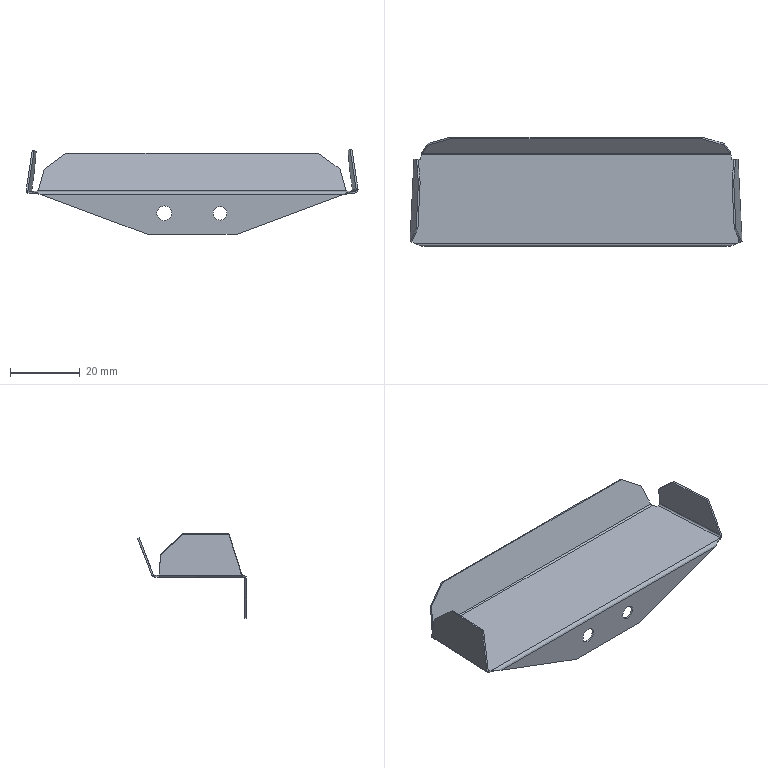Part | SolidWorks | features BaseBody 1 | 1 solid | 54 faces | box 95.197 x 31.29 x 24.218 mm | volume 2286 mm3 | plane 32 | cylinder 14 | spline 8 | commonest cylinder face diameters 1 x6 2 x4 3.922 x2 4.202 x2